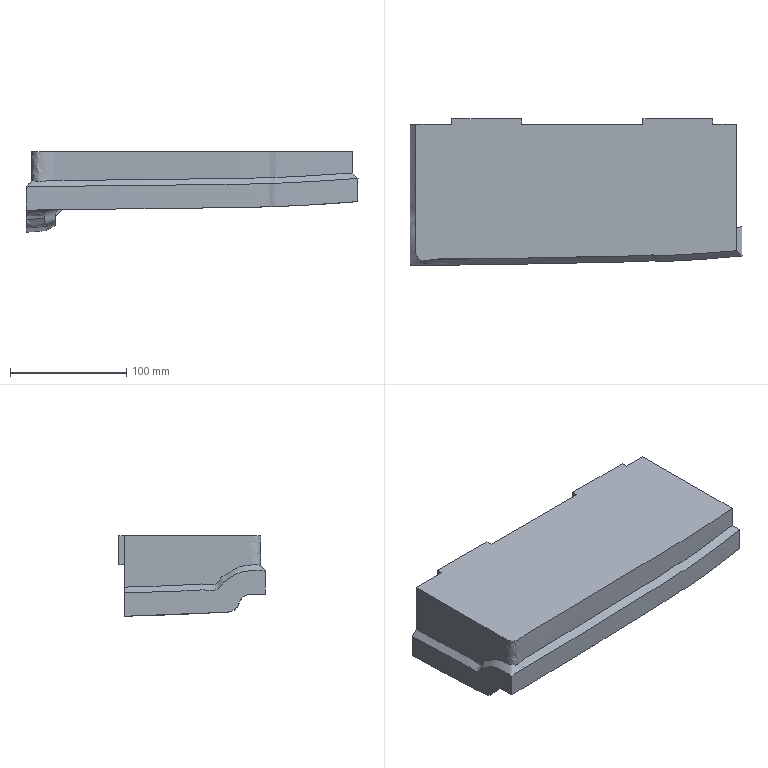Part | NX | features solid 2 | 1 solid | 44 faces | box 285 x 125.888 x 69.1 mm | volume 1066718 mm3 | plane 23 | spline 16 | cylinder 5 | commonest cylinder face diameters 30 x5